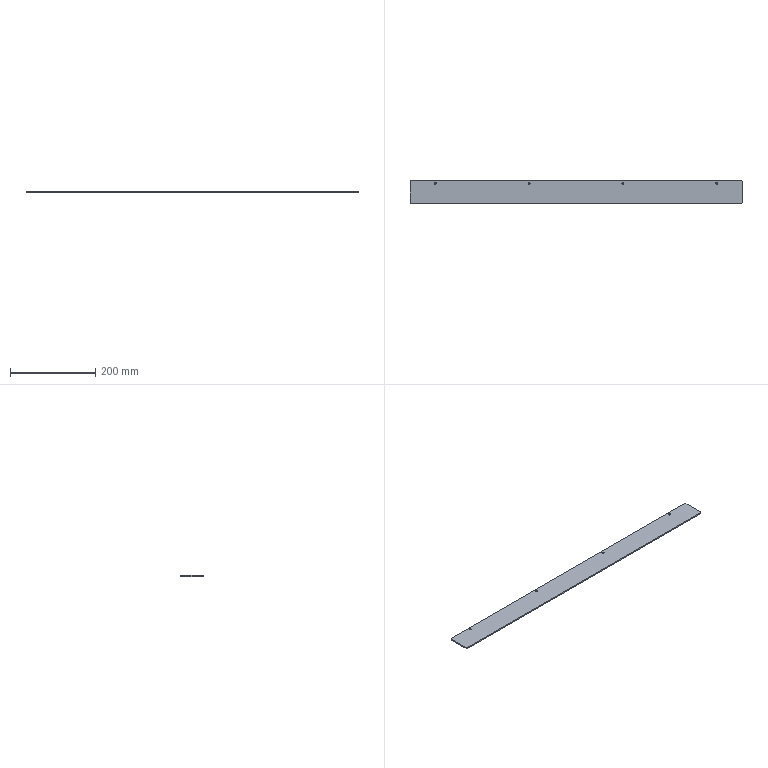Part | NX | features BREP 1 | 1 solid | 26 faces | box 778 x 53 x 3 mm | volume 123272 mm3 | plane 10 | cone 8 | cylinder 8 | commonest cylinder face diameters 4.8 x8
STEP:
#1=CARTESIAN_POINT('',(389.,24.5,3.));
#2=VERTEX_POINT('',#1);
#3=CARTESIAN_POINT('',(387.,26.5,3.));
#4=VERTEX_POINT('',#3);
#5=CARTESIAN_POINT('',(206.75,206.75,3.));
#6=DIRECTION('',(-0.7071,0.7071,0.));
#7=VECTOR('',#6,1000.);
#8=LINE('',#5,#7);
#9=EDGE_CURVE('',#2,#4,#8,.T.);
#10=ORIENTED_EDGE('',*,*,#9,.F.);
#11=CARTESIAN_POINT('',(389.,24.5,0.));
#12=VERTEX_POINT('',#11);
#13=CARTESIAN_POINT('',(389.,24.5,3.));
#14=DIRECTION('',(0.,0.,1.));
#15=VECTOR('',#14,1000.);
#16=LINE('',#13,#15);
#17=EDGE_CURVE('',#12,#2,#16,.T.);
#18=ORIENTED_EDGE('',*,*,#17,.F.);
#19=CARTESIAN_POINT('',(387.,26.5,0.));
#20=VERTEX_POINT('',#19);
#21=CARTESIAN_POINT('',(387.,26.5,0.));
#22=DIRECTION('',(0.7071,-0.7071,0.));
#23=VECTOR('',#22,1000.);
#24=LINE('',#21,#23);
#25=EDGE_CURVE('',#20,#12,#24,.T.);
#26=ORIENTED_EDGE('',*,*,#25,.F.);
#27=CARTESIAN_POINT('',(387.,26.5,3.));
#28=DIRECTION('',(0.,0.,-1.));
#29=VECTOR('',#28,1000.);
#30=LINE('',#27,#29);
#31=EDGE_CURVE('',#4,#20,#30,.T.);
#32=ORIENTED_EDGE('',*,*,#31,.F.);
#33=EDGE_LOOP('',(#10,#18,#26,#32));
#34=FACE_BOUND('',#33,.T.);
#35=CARTESIAN_POINT('',(387.,26.5,3.));
#36=DIRECTION('',(-0.7071,-0.7071,0.));
#37=DIRECTION('',(0.,0.,-1.));
#38=AXIS2_PLACEMENT_3D('',#35,#36,#37);
#39=PLANE('',#38);
#40=ADVANCED_FACE('',(#34),#39,.F.);
#41=CARTESIAN_POINT('',(387.,-26.5,3.));
#42=VERTEX_POINT('',#41);
#43=CARTESIAN_POINT('',(389.,-24.5,3.));
#44=VERTEX_POINT('',#43);
#45=CARTESIAN_POINT('',(206.75,-206.75,3.));
#46=DIRECTION('',(0.7071,0.7071,0.));
#47=VECTOR('',#46,1000.);
#48=LINE('',#45,#47);
#49=EDGE_CURVE('',#42,#44,#48,.T.);
#50=ORIENTED_EDGE('',*,*,#49,.F.);
#51=CARTESIAN_POINT('',(387.,-26.5,0.));
#52=VERTEX_POINT('',#51);
#53=CARTESIAN_POINT('',(387.,-26.5,3.));
#54=DIRECTION('',(0.,0.,1.));
#55=VECTOR('',#54,1000.);
#56=LINE('',#53,#55);
#57=EDGE_CURVE('',#52,#42,#56,.T.);
#58=ORIENTED_EDGE('',*,*,#57,.F.);
#59=CARTESIAN_POINT('',(389.,-24.5,0.));
#60=VERTEX_POINT('',#59);
#61=CARTESIAN_POINT('',(389.,-24.5,0.));
#62=DIRECTION('',(-0.7071,-0.7071,0.));
#63=VECTOR('',#62,1000.);
#64=LINE('',#61,#63);
#65=EDGE_CURVE('',#60,#52,#64,.T.);
#66=ORIENTED_EDGE('',*,*,#65,.F.);
#67=CARTESIAN_POINT('',(389.,-24.5,3.));
#68=DIRECTION('',(0.,0.,-1.));
#69=VECTOR('',#68,1000.);
#70=LINE('',#67,#69);
#71=EDGE_CURVE('',#44,#60,#70,.T.);
#72=ORIENTED_EDGE('',*,*,#71,.F.);
#73=EDGE_LOOP('',(#50,#58,#66,#72));
#74=FACE_BOUND('',#73,.T.);
#75=CARTESIAN_POINT('',(389.,-24.5,3.));
#76=DIRECTION('',(-0.7071,0.7071,0.));
#77=DIRECTION('',(0.,0.,-1.));
#78=AXIS2_PLACEMENT_3D('',#75,#76,#77);
#79=PLANE('',#78);
#80=ADVANCED_FACE('',(#74),#79,.F.);
#81=CARTESIAN_POINT('',(-387.,26.5,3.));
#82=VERTEX_POINT('',#81);
#83=CARTESIAN_POINT('',(-389.,24.5,3.));
#84=VERTEX_POINT('',#83);
#85=CARTESIAN_POINT('',(-206.75,206.75,3.));
#86=DIRECTION('',(-0.7071,-0.7071,0.));
#87=VECTOR('',#86,1000.);
#88=LINE('',#85,#87);
#89=EDGE_CURVE('',#82,#84,#88,.T.);
#90=ORIENTED_EDGE('',*,*,#89,.F.);
#91=CARTESIAN_POINT('',(-387.,26.5,0.));
#92=VERTEX_POINT('',#91);
#93=CARTESIAN_POINT('',(-387.,26.5,3.));
#94=DIRECTION('',(0.,0.,1.));
#95=VECTOR('',#94,1000.);
#96=LINE('',#93,#95);
#97=EDGE_CURVE('',#92,#82,#96,.T.);
#98=ORIENTED_EDGE('',*,*,#97,.F.);
#99=CARTESIAN_POINT('',(-389.,24.5,0.));
#100=VERTEX_POINT('',#99);
#101=CARTESIAN_POINT('',(-389.,24.5,0.));
#102=DIRECTION('',(0.7071,0.7071,0.));
#103=VECTOR('',#102,1000.);
#104=LINE('',#101,#103);
#105=EDGE_CURVE('',#100,#92,#104,.T.);
#106=ORIENTED_EDGE('',*,*,#105,.F.);
#107=CARTESIAN_POINT('',(-389.,24.5,3.));
#108=DIRECTION('',(0.,0.,-1.));
#109=VECTOR('',#108,1000.);
#110=LINE('',#107,#109);
#111=EDGE_CURVE('',#84,#100,#110,.T.);
#112=ORIENTED_EDGE('',*,*,#111,.F.);
#113=EDGE_LOOP('',(#90,#98,#106,#112));
#114=FACE_BOUND('',#113,.T.);
#115=CARTESIAN_POINT('',(-389.,24.5,3.));
#116=DIRECTION('',(0.7071,-0.7071,0.));
#117=DIRECTION('',(0.,0.,-1.));
#118=AXIS2_PLACEMENT_3D('',#115,#116,#117);
#119=PLANE('',#118);
#120=ADVANCED_FACE('',(#114),#119,.F.);
#121=CARTESIAN_POINT('',(-389.,-24.5,3.));
#122=VERTEX_POINT('',#121);
#123=CARTESIAN_POINT('',(-387.,-26.5,3.));
#124=VERTEX_POINT('',#123);
#125=CARTESIAN_POINT('',(-206.75,-206.75,3.));
#126=DIRECTION('',(0.7071,-0.7071,0.));
#127=VECTOR('',#126,1000.);
#128=LINE('',#125,#127);
#129=EDGE_CURVE('',#122,#124,#128,.T.);
#130=ORIENTED_EDGE('',*,*,#129,.F.);
#131=CARTESIAN_POINT('',(-389.,-24.5,0.));
#132=VERTEX_POINT('',#131);
#133=CARTESIAN_POINT('',(-389.,-24.5,3.));
#134=DIRECTION('',(0.,0.,1.));
#135=VECTOR('',#134,1000.);
#136=LINE('',#133,#135);
#137=EDGE_CURVE('',#132,#122,#136,.T.);
#138=ORIENTED_EDGE('',*,*,#137,.F.);
#139=CARTESIAN_POINT('',(-387.,-26.5,0.));
#140=VERTEX_POINT('',#139);
#141=CARTESIAN_POINT('',(-387.,-26.5,0.));
#142=DIRECTION('',(-0.7071,0.7071,0.));
#143=VECTOR('',#142,1000.);
#144=LINE('',#141,#143);
#145=EDGE_CURVE('',#140,#132,#144,.T.);
#146=ORIENTED_EDGE('',*,*,#145,.F.);
#147=CARTESIAN_POINT('',(-387.,-26.5,3.));
#148=DIRECTION('',(0.,0.,-1.));
#149=VECTOR('',#148,1000.);
#150=LINE('',#147,#149);
#151=EDGE_CURVE('',#124,#140,#150,.T.);
#152=ORIENTED_EDGE('',*,*,#151,.F.);
#153=EDGE_LOOP('',(#130,#138,#146,#152));
#154=FACE_BOUND('',#153,.T.);
#155=CARTESIAN_POINT('',(-387.,-26.5,3.));
#156=DIRECTION('',(0.7071,0.7071,0.));
#157=DIRECTION('',(0.,0.,-1.));
#158=AXIS2_PLACEMENT_3D('',#155,#156,#157);
#159=PLANE('',#158);
#160=ADVANCED_FACE('',(#154),#159,.F.);
#161=CARTESIAN_POINT('',(332.4,20.5,2.19));
#162=VERTEX_POINT('',#161);
#163=CARTESIAN_POINT('',(334.59,20.5,0.));
#164=VERTEX_POINT('',#163);
#165=CARTESIAN_POINT('',(334.59,20.5,0.));
#166=DIRECTION('',(0.7071,0.,-0.7071));
#167=VECTOR('',#166,1000.);
#168=LINE('',#165,#167);
#169=EDGE_CURVE('',#162,#164,#168,.T.);
#170=ORIENTED_EDGE('',*,*,#169,.F.);
#171=CARTESIAN_POINT('',(327.6,20.5,2.19));
#172=VERTEX_POINT('',#171);
#173=CARTESIAN_POINT('',(330.,20.5,2.19));
#174=DIRECTION('',(0.,0.,-1.));
#175=DIRECTION('',(-1.,0.,0.));
#176=AXIS2_PLACEMENT_3D('',#173,#174,#175);
#177=CIRCLE('',#176,2.4);
#178=EDGE_CURVE('',#172,#162,#177,.T.);
#179=ORIENTED_EDGE('',*,*,#178,.F.);
#180=CARTESIAN_POINT('',(325.41,20.5,0.));
#181=VERTEX_POINT('',#180);
#182=CARTESIAN_POINT('',(325.41,20.5,0.));
#183=DIRECTION('',(-0.7071,0.,-0.7071));
#184=VECTOR('',#183,1000.);
#185=LINE('',#182,#184);
#186=EDGE_CURVE('',#172,#181,#185,.T.);
#187=ORIENTED_EDGE('',*,*,#186,.T.);
#188=CARTESIAN_POINT('',(330.,20.5,0.));
#189=DIRECTION('',(0.,0.,-1.));
#190=DIRECTION('',(-1.,0.,0.));
#191=AXIS2_PLACEMENT_3D('',#188,#189,#190);
#192=CIRCLE('',#191,4.59);
#193=EDGE_CURVE('',#181,#164,#192,.T.);
#194=ORIENTED_EDGE('',*,*,#193,.T.);
#195=EDGE_LOOP('',(#170,#179,#187,#194));
#196=FACE_BOUND('',#195,.T.);
#197=CARTESIAN_POINT('',(330.,20.5,0.));
#198=DIRECTION('',(0.,0.,-1.));
#199=DIRECTION('',(-1.,0.,0.));
#200=AXIS2_PLACEMENT_3D('',#197,#198,#199);
#201=CONICAL_SURFACE('',#200,4.59,0.7854);
#202=ADVANCED_FACE('',(#196),#201,.F.);
#203=CARTESIAN_POINT('',(332.4,20.5,3.));
#204=VERTEX_POINT('',#203);
#205=CARTESIAN_POINT('',(332.4,20.5,0.));
#206=DIRECTION('',(0.,0.,-1.));
#207=VECTOR('',#206,1000.);
#208=LINE('',#205,#207);
#209=EDGE_CURVE('',#204,#162,#208,.T.);
#210=ORIENTED_EDGE('',*,*,#209,.F.);
#211=CARTESIAN_POINT('',(327.6,20.5,3.));
#212=VERTEX_POINT('',#211);
#213=CARTESIAN_POINT('',(330.,20.5,3.));
#214=DIRECTION('',(0.,0.,-1.));
#215=DIRECTION('',(-1.,0.,0.));
#216=AXIS2_PLACEMENT_3D('',#213,#214,#215);
#217=CIRCLE('',#216,2.4);
#218=EDGE_CURVE('',#212,#204,#217,.T.);
#219=ORIENTED_EDGE('',*,*,#218,.F.);
#220=CARTESIAN_POINT('',(327.6,20.5,0.));
#221=DIRECTION('',(0.,0.,-1.));
#222=VECTOR('',#221,1000.);
#223=LINE('',#220,#222);
#224=EDGE_CURVE('',#212,#172,#223,.T.);
#225=ORIENTED_EDGE('',*,*,#224,.T.);
#226=ORIENTED_EDGE('',*,*,#178,.T.);
#227=EDGE_LOOP('',(#210,#219,#225,#226));
#228=FACE_BOUND('',#227,.T.);
#229=CARTESIAN_POINT('',(330.,20.5,0.));
#230=DIRECTION('',(0.,0.,-1.));
#231=DIRECTION('',(-1.,0.,0.));
#232=AXIS2_PLACEMENT_3D('',#229,#230,#231);
#233=CYLINDRICAL_SURFACE('',#232,2.4);
#234=ADVANCED_FACE('',(#228),#233,.F.);
#235=CARTESIAN_POINT('',(112.4,20.5,2.19));
#236=VERTEX_POINT('',#235);
#237=CARTESIAN_POINT('',(114.59,20.5,0.));
#238=VERTEX_POINT('',#237);
#239=CARTESIAN_POINT('',(114.59,20.5,0.));
#240=DIRECTION('',(0.7071,0.,-0.7071));
#241=VECTOR('',#240,1000.);
#242=LINE('',#239,#241);
#243=EDGE_CURVE('',#236,#238,#242,.T.);
#244=ORIENTED_EDGE('',*,*,#243,.F.);
#245=CARTESIAN_POINT('',(107.6,20.5,2.19));
#246=VERTEX_POINT('',#245);
#247=CARTESIAN_POINT('',(110.,20.5,2.19));
#248=DIRECTION('',(0.,0.,-1.));
#249=DIRECTION('',(-1.,0.,0.));
#250=AXIS2_PLACEMENT_3D('',#247,#248,#249);
#251=CIRCLE('',#250,2.4);
#252=EDGE_CURVE('',#246,#236,#251,.T.);
#253=ORIENTED_EDGE('',*,*,#252,.F.);
#254=CARTESIAN_POINT('',(105.41,20.5,0.));
#255=VERTEX_POINT('',#254);
#256=CARTESIAN_POINT('',(105.41,20.5,0.));
#257=DIRECTION('',(-0.7071,0.,-0.7071));
#258=VECTOR('',#257,1000.);
#259=LINE('',#256,#258);
#260=EDGE_CURVE('',#246,#255,#259,.T.);
#261=ORIENTED_EDGE('',*,*,#260,.T.);
#262=CARTESIAN_POINT('',(110.,20.5,0.));
#263=DIRECTION('',(0.,0.,-1.));
#264=DIRECTION('',(-1.,0.,0.));
#265=AXIS2_PLACEMENT_3D('',#262,#263,#264);
#266=CIRCLE('',#265,4.59);
#267=EDGE_CURVE('',#255,#238,#266,.T.);
#268=ORIENTED_EDGE('',*,*,#267,.T.);
#269=EDGE_LOOP('',(#244,#253,#261,#268));
#270=FACE_BOUND('',#269,.T.);
#271=CARTESIAN_POINT('',(110.,20.5,0.));
#272=DIRECTION('',(0.,0.,-1.));
#273=DIRECTION('',(-1.,0.,0.));
#274=AXIS2_PLACEMENT_3D('',#271,#272,#273);
#275=CONICAL_SURFACE('',#274,4.59,0.7854);
#276=ADVANCED_FACE('',(#270),#275,.F.);
#277=CARTESIAN_POINT('',(112.4,20.5,3.));
#278=VERTEX_POINT('',#277);
#279=CARTESIAN_POINT('',(112.4,20.5,0.));
#280=DIRECTION('',(0.,0.,-1.));
#281=VECTOR('',#280,1000.);
#282=LINE('',#279,#281);
#283=EDGE_CURVE('',#278,#236,#282,.T.);
#284=ORIENTED_EDGE('',*,*,#283,.F.);
#285=CARTESIAN_POINT('',(107.6,20.5,3.));
#286=VERTEX_POINT('',#285);
#287=CARTESIAN_POINT('',(110.,20.5,3.));
#288=DIRECTION('',(0.,0.,-1.));
#289=DIRECTION('',(-1.,0.,0.));
#290=AXIS2_PLACEMENT_3D('',#287,#288,#289);
#291=CIRCLE('',#290,2.4);
#292=EDGE_CURVE('',#286,#278,#291,.T.);
#293=ORIENTED_EDGE('',*,*,#292,.F.);
#294=CARTESIAN_POINT('',(107.6,20.5,0.));
#295=DIRECTION('',(0.,0.,-1.));
#296=VECTOR('',#295,1000.);
#297=LINE('',#294,#296);
#298=EDGE_CURVE('',#286,#246,#297,.T.);
#299=ORIENTED_EDGE('',*,*,#298,.T.);
#300=ORIENTED_EDGE('',*,*,#252,.T.);
#301=EDGE_LOOP('',(#284,#293,#299,#300));
#302=FACE_BOUND('',#301,.T.);
#303=CARTESIAN_POINT('',(110.,20.5,0.));
#304=DIRECTION('',(0.,0.,-1.));
#305=DIRECTION('',(-1.,0.,0.));
#306=AXIS2_PLACEMENT_3D('',#303,#304,#305);
#307=CYLINDRICAL_SURFACE('',#306,2.4);
#308=ADVANCED_FACE('',(#302),#307,.F.);
#309=CARTESIAN_POINT('',(-107.6,20.5,2.19));
#310=VERTEX_POINT('',#309);
#311=CARTESIAN_POINT('',(-105.41,20.5,0.));
#312=VERTEX_POINT('',#311);
#313=CARTESIAN_POINT('',(-105.41,20.5,0.));
#314=DIRECTION('',(0.7071,0.,-0.7071));
#315=VECTOR('',#314,1000.);
#316=LINE('',#313,#315);
#317=EDGE_CURVE('',#310,#312,#316,.T.);
#318=ORIENTED_EDGE('',*,*,#317,.F.);
#319=CARTESIAN_POINT('',(-112.4,20.5,2.19));
#320=VERTEX_POINT('',#319);
#321=CARTESIAN_POINT('',(-110.,20.5,2.19));
#322=DIRECTION('',(0.,0.,-1.));
#323=DIRECTION('',(-1.,0.,0.));
#324=AXIS2_PLACEMENT_3D('',#321,#322,#323);
#325=CIRCLE('',#324,2.4);
#326=EDGE_CURVE('',#320,#310,#325,.T.);
#327=ORIENTED_EDGE('',*,*,#326,.F.);
#328=CARTESIAN_POINT('',(-114.59,20.5,0.));
#329=VERTEX_POINT('',#328);
#330=CARTESIAN_POINT('',(-114.59,20.5,0.));
#331=DIRECTION('',(-0.7071,0.,-0.7071));
#332=VECTOR('',#331,1000.);
#333=LINE('',#330,#332);
#334=EDGE_CURVE('',#320,#329,#333,.T.);
#335=ORIENTED_EDGE('',*,*,#334,.T.);
#336=CARTESIAN_POINT('',(-110.,20.5,0.));
#337=DIRECTION('',(0.,0.,-1.));
#338=DIRECTION('',(-1.,0.,0.));
#339=AXIS2_PLACEMENT_3D('',#336,#337,#338);
#340=CIRCLE('',#339,4.59);
#341=EDGE_CURVE('',#329,#312,#340,.T.);
#342=ORIENTED_EDGE('',*,*,#341,.T.);
#343=EDGE_LOOP('',(#318,#327,#335,#342));
#344=FACE_BOUND('',#343,.T.);
#345=CARTESIAN_POINT('',(-110.,20.5,0.));
#346=DIRECTION('',(0.,0.,-1.));
#347=DIRECTION('',(-1.,0.,0.));
#348=AXIS2_PLACEMENT_3D('',#345,#346,#347);
#349=CONICAL_SURFACE('',#348,4.59,0.7854);
#350=ADVANCED_FACE('',(#344),#349,.F.);
#351=CARTESIAN_POINT('',(-107.6,20.5,3.));
#352=VERTEX_POINT('',#351);
#353=CARTESIAN_POINT('',(-107.6,20.5,0.));
#354=DIRECTION('',(0.,0.,-1.));
#355=VECTOR('',#354,1000.);
#356=LINE('',#353,#355);
#357=EDGE_CURVE('',#352,#310,#356,.T.);
#358=ORIENTED_EDGE('',*,*,#357,.F.);
#359=CARTESIAN_POINT('',(-112.4,20.5,3.));
#360=VERTEX_POINT('',#359);
#361=CARTESIAN_POINT('',(-110.,20.5,3.));
#362=DIRECTION('',(0.,0.,-1.));
#363=DIRECTION('',(-1.,0.,0.));
#364=AXIS2_PLACEMENT_3D('',#361,#362,#363);
#365=CIRCLE('',#364,2.4);
#366=EDGE_CURVE('',#360,#352,#365,.T.);
#367=ORIENTED_EDGE('',*,*,#366,.F.);
#368=CARTESIAN_POINT('',(-112.4,20.5,0.));
#369=DIRECTION('',(0.,0.,-1.));
#370=VECTOR('',#369,1000.);
#371=LINE('',#368,#370);
#372=EDGE_CURVE('',#360,#320,#371,.T.);
#373=ORIENTED_EDGE('',*,*,#372,.T.);
#374=ORIENTED_EDGE('',*,*,#326,.T.);
#375=EDGE_LOOP('',(#358,#367,#373,#374));
#376=FACE_BOUND('',#375,.T.);
#377=CARTESIAN_POINT('',(-110.,20.5,0.));
#378=DIRECTION('',(0.,0.,-1.));
#379=DIRECTION('',(-1.,0.,0.));
#380=AXIS2_PLACEMENT_3D('',#377,#378,#379);
#381=CYLINDRICAL_SURFACE('',#380,2.4);
#382=ADVANCED_FACE('',(#376),#381,.F.);
#383=CARTESIAN_POINT('',(-327.6,20.5,2.19));
#384=VERTEX_POINT('',#383);
#385=CARTESIAN_POINT('',(-325.41,20.5,0.));
#386=VERTEX_POINT('',#385);
#387=CARTESIAN_POINT('',(-325.41,20.5,0.));
#388=DIRECTION('',(0.7071,0.,-0.7071));
#389=VECTOR('',#388,1000.);
#390=LINE('',#387,#389);
#391=EDGE_CURVE('',#384,#386,#390,.T.);
#392=ORIENTED_EDGE('',*,*,#391,.F.);
#393=CARTESIAN_POINT('',(-332.4,20.5,2.19));
#394=VERTEX_POINT('',#393);
#395=CARTESIAN_POINT('',(-330.,20.5,2.19));
#396=DIRECTION('',(0.,0.,-1.));
#397=DIRECTION('',(-1.,0.,0.));
#398=AXIS2_PLACEMENT_3D('',#395,#396,#397);
#399=CIRCLE('',#398,2.4);
#400=EDGE_CURVE('',#394,#384,#399,.T.);
#401=ORIENTED_EDGE('',*,*,#400,.F.);
#402=CARTESIAN_POINT('',(-334.59,20.5,0.));
#403=VERTEX_POINT('',#402);
#404=CARTESIAN_POINT('',(-334.59,20.5,0.));
#405=DIRECTION('',(-0.7071,0.,-0.7071));
#406=VECTOR('',#405,1000.);
#407=LINE('',#404,#406);
#408=EDGE_CURVE('',#394,#403,#407,.T.);
#409=ORIENTED_EDGE('',*,*,#408,.T.);
#410=CARTESIAN_POINT('',(-330.,20.5,0.));
#411=DIRECTION('',(0.,0.,-1.));
#412=DIRECTION('',(-1.,0.,0.));
#413=AXIS2_PLACEMENT_3D('',#410,#411,#412);
#414=CIRCLE('',#413,4.59);
#415=EDGE_CURVE('',#403,#386,#414,.T.);
#416=ORIENTED_EDGE('',*,*,#415,.T.);
#417=EDGE_LOOP('',(#392,#401,#409,#416));
#418=FACE_BOUND('',#417,.T.);
#419=CARTESIAN_POINT('',(-330.,20.5,0.));
#420=DIRECTION('',(0.,0.,-1.));
#421=DIRECTION('',(-1.,0.,0.));
#422=AXIS2_PLACEMENT_3D('',#419,#420,#421);
#423=CONICAL_SURFACE('',#422,4.59,0.7854);
#424=ADVANCED_FACE('',(#418),#423,.F.);
#425=CARTESIAN_POINT('',(-327.6,20.5,3.));
#426=VERTEX_POINT('',#425);
#427=CARTESIAN_POINT('',(-327.6,20.5,0.));
#428=DIRECTION('',(0.,0.,-1.));
#429=VECTOR('',#428,1000.);
#430=LINE('',#427,#429);
#431=EDGE_CURVE('',#426,#384,#430,.T.);
#432=ORIENTED_EDGE('',*,*,#431,.F.);
#433=CARTESIAN_POINT('',(-332.4,20.5,3.));
#434=VERTEX_POINT('',#433);
#435=CARTESIAN_POINT('',(-330.,20.5,3.));
#436=DIRECTION('',(0.,0.,-1.));
#437=DIRECTION('',(-1.,0.,0.));
#438=AXIS2_PLACEMENT_3D('',#435,#436,#437);
#439=CIRCLE('',#438,2.4);
#440=EDGE_CURVE('',#434,#426,#439,.T.);
#441=ORIENTED_EDGE('',*,*,#440,.F.);
#442=CARTESIAN_POINT('',(-332.4,20.5,0.));
#443=DIRECTION('',(0.,0.,-1.));
#444=VECTOR('',#443,1000.);
#445=LINE('',#442,#444);
#446=EDGE_CURVE('',#434,#394,#445,.T.);
#447=ORIENTED_EDGE('',*,*,#446,.T.);
#448=ORIENTED_EDGE('',*,*,#400,.T.);
#449=EDGE_LOOP('',(#432,#441,#447,#448));
#450=FACE_BOUND('',#449,.T.);
#451=CARTESIAN_POINT('',(-330.,20.5,0.));
#452=DIRECTION('',(0.,0.,-1.));
#453=DIRECTION('',(-1.,0.,0.));
#454=AXIS2_PLACEMENT_3D('',#451,#452,#453);
#455=CYLINDRICAL_SURFACE('',#454,2.4);
#456=ADVANCED_FACE('',(#450),#455,.F.);
#457=CARTESIAN_POINT('',(389.,-26.5,0.));
#458=DIRECTION('',(1.,0.,0.));
#459=VECTOR('',#458,1000.);
#460=LINE('',#457,#459);
#461=EDGE_CURVE('',#140,#52,#460,.T.);
#462=ORIENTED_EDGE('',*,*,#461,.F.);
#463=ORIENTED_EDGE('',*,*,#145,.T.);
#464=CARTESIAN_POINT('',(-389.,-26.5,0.));
#465=DIRECTION('',(0.,-1.,0.));
#466=VECTOR('',#465,1000.);
#467=LINE('',#464,#466);
#468=EDGE_CURVE('',#100,#132,#467,.T.);
#469=ORIENTED_EDGE('',*,*,#468,.F.);
#470=ORIENTED_EDGE('',*,*,#105,.T.);
#471=CARTESIAN_POINT('',(389.,26.5,0.));
#472=DIRECTION('',(-1.,0.,0.));
#473=VECTOR('',#472,1000.);
#474=LINE('',#471,#473);
#475=EDGE_CURVE('',#20,#92,#474,.T.);
#476=ORIENTED_EDGE('',*,*,#475,.F.);
#477=ORIENTED_EDGE('',*,*,#25,.T.);
#478=CARTESIAN_POINT('',(389.,-26.5,0.));
#479=DIRECTION('',(0.,1.,0.));
#480=VECTOR('',#479,1000.);
#481=LINE('',#478,#480);
#482=EDGE_CURVE('',#60,#12,#481,.T.);
#483=ORIENTED_EDGE('',*,*,#482,.F.);
#484=ORIENTED_EDGE('',*,*,#65,.T.);
#485=EDGE_LOOP('',(#462,#463,#469,#470,#476,#477,#483,#484));
#486=FACE_BOUND('',#485,.T.);
#487=ORIENTED_EDGE('',*,*,#415,.F.);
#488=CARTESIAN_POINT('',(-330.,20.5,0.));
#489=DIRECTION('',(0.,0.,-1.));
#490=DIRECTION('',(-1.,0.,0.));
#491=AXIS2_PLACEMENT_3D('',#488,#489,#490);
#492=CIRCLE('',#491,4.59);
#493=EDGE_CURVE('',#386,#403,#492,.T.);
#494=ORIENTED_EDGE('',*,*,#493,.F.);
#495=EDGE_LOOP('',(#487,#494));
#496=FACE_BOUND('',#495,.T.);
#497=ORIENTED_EDGE('',*,*,#341,.F.);
#498=CARTESIAN_POINT('',(-110.,20.5,0.));
#499=DIRECTION('',(0.,0.,-1.));
#500=DIRECTION('',(-1.,0.,0.));
#501=AXIS2_PLACEMENT_3D('',#498,#499,#500);
#502=CIRCLE('',#501,4.59);
#503=EDGE_CURVE('',#312,#329,#502,.T.);
#504=ORIENTED_EDGE('',*,*,#503,.F.);
#505=EDGE_LOOP('',(#497,#504));
#506=FACE_BOUND('',#505,.T.);
#507=ORIENTED_EDGE('',*,*,#267,.F.);
#508=CARTESIAN_POINT('',(110.,20.5,0.));
#509=DIRECTION('',(0.,0.,-1.));
#510=DIRECTION('',(-1.,0.,0.));
#511=AXIS2_PLACEMENT_3D('',#508,#509,#510);
#512=CIRCLE('',#511,4.59);
#513=EDGE_CURVE('',#238,#255,#512,.T.);
#514=ORIENTED_EDGE('',*,*,#513,.F.);
#515=EDGE_LOOP('',(#507,#514));
#516=FACE_BOUND('',#515,.T.);
#517=ORIENTED_EDGE('',*,*,#193,.F.);
#518=CARTESIAN_POINT('',(330.,20.5,0.));
#519=DIRECTION('',(0.,0.,-1.));
#520=DIRECTION('',(-1.,0.,0.));
#521=AXIS2_PLACEMENT_3D('',#518,#519,#520);
#522=CIRCLE('',#521,4.59);
#523=EDGE_CURVE('',#164,#181,#522,.T.);
#524=ORIENTED_EDGE('',*,*,#523,.F.);
#525=EDGE_LOOP('',(#517,#524));
#526=FACE_BOUND('',#525,.T.);
#527=CARTESIAN_POINT('',(0.,0.,0.));
#528=DIRECTION('',(0.,0.,1.));
#529=DIRECTION('',(1.,0.,0.));
#530=AXIS2_PLACEMENT_3D('',#527,#528,#529);
#531=PLANE('',#530);
#532=ADVANCED_FACE('',(#486,#496,#506,#516,#526),#531,.F.);
#533=CARTESIAN_POINT('',(-389.,-26.5,3.));
#534=DIRECTION('',(0.,-1.,0.));
#535=VECTOR('',#534,1000.);
#536=LINE('',#533,#535);
#537=EDGE_CURVE('',#84,#122,#536,.T.);
#538=ORIENTED_EDGE('',*,*,#537,.T.);
#539=ORIENTED_EDGE('',*,*,#129,.T.);
#540=CARTESIAN_POINT('',(389.,-26.5,3.));
#541=DIRECTION('',(1.,0.,0.));
#542=VECTOR('',#541,1000.);
#543=LINE('',#540,#542);
#544=EDGE_CURVE('',#124,#42,#543,.T.);
#545=ORIENTED_EDGE('',*,*,#544,.T.);
#546=ORIENTED_EDGE('',*,*,#49,.T.);
#547=CARTESIAN_POINT('',(389.,-26.5,3.));
#548=DIRECTION('',(0.,1.,0.));
#549=VECTOR('',#548,1000.);
#550=LINE('',#547,#549);
#551=EDGE_CURVE('',#44,#2,#550,.T.);
#552=ORIENTED_EDGE('',*,*,#551,.T.);
#553=ORIENTED_EDGE('',*,*,#9,.T.);
#554=CARTESIAN_POINT('',(389.,26.5,3.));
#555=DIRECTION('',(-1.,0.,0.));
#556=VECTOR('',#555,1000.);
#557=LINE('',#554,#556);
#558=EDGE_CURVE('',#4,#82,#557,.T.);
#559=ORIENTED_EDGE('',*,*,#558,.T.);
#560=ORIENTED_EDGE('',*,*,#89,.T.);
#561=EDGE_LOOP('',(#538,#539,#545,#546,#552,#553,#559,#560));
#562=FACE_BOUND('',#561,.T.);
#563=ORIENTED_EDGE('',*,*,#440,.T.);
#564=CARTESIAN_POINT('',(-330.,20.5,3.));
#565=DIRECTION('',(0.,0.,-1.));
#566=DIRECTION('',(-1.,0.,0.));
#567=AXIS2_PLACEMENT_3D('',#564,#565,#566);
#568=CIRCLE('',#567,2.4);
#569=EDGE_CURVE('',#426,#434,#568,.T.);
#570=ORIENTED_EDGE('',*,*,#569,.T.);
#571=EDGE_LOOP('',(#563,#570));
#572=FACE_BOUND('',#571,.T.);
#573=ORIENTED_EDGE('',*,*,#366,.T.);
#574=CARTESIAN_POINT('',(-110.,20.5,3.));
#575=DIRECTION('',(0.,0.,-1.));
#576=DIRECTION('',(-1.,0.,0.));
#577=AXIS2_PLACEMENT_3D('',#574,#575,#576);
#578=CIRCLE('',#577,2.4);
#579=EDGE_CURVE('',#352,#360,#578,.T.);
#580=ORIENTED_EDGE('',*,*,#579,.T.);
#581=EDGE_LOOP('',(#573,#580));
#582=FACE_BOUND('',#581,.T.);
#583=ORIENTED_EDGE('',*,*,#292,.T.);
#584=CARTESIAN_POINT('',(110.,20.5,3.));
#585=DIRECTION('',(0.,0.,-1.));
#586=DIRECTION('',(-1.,0.,0.));
#587=AXIS2_PLACEMENT_3D('',#584,#585,#586);
#588=CIRCLE('',#587,2.4);
#589=EDGE_CURVE('',#278,#286,#588,.T.);
#590=ORIENTED_EDGE('',*,*,#589,.T.);
#591=EDGE_LOOP('',(#583,#590));
#592=FACE_BOUND('',#591,.T.);
#593=ORIENTED_EDGE('',*,*,#218,.T.);
#594=CARTESIAN_POINT('',(330.,20.5,3.));
#595=DIRECTION('',(0.,0.,-1.));
#596=DIRECTION('',(-1.,0.,0.));
#597=AXIS2_PLACEMENT_3D('',#594,#595,#596);
#598=CIRCLE('',#597,2.4);
#599=EDGE_CURVE('',#204,#212,#598,.T.);
#600=ORIENTED_EDGE('',*,*,#599,.T.);
#601=EDGE_LOOP('',(#593,#600));
#602=FACE_BOUND('',#601,.T.);
#603=CARTESIAN_POINT('',(0.,0.,3.));
#604=DIRECTION('',(0.,0.,1.));
#605=DIRECTION('',(1.,0.,0.));
#606=AXIS2_PLACEMENT_3D('',#603,#604,#605);
#607=PLANE('',#606);
#608=ADVANCED_FACE('',(#562,#572,#582,#592,#602),#607,.T.);
#609=ORIENTED_EDGE('',*,*,#475,.T.);
#610=ORIENTED_EDGE('',*,*,#97,.T.);
#611=ORIENTED_EDGE('',*,*,#558,.F.);
#612=ORIENTED_EDGE('',*,*,#31,.T.);
#613=EDGE_LOOP('',(#609,#610,#611,#612));
#614=FACE_BOUND('',#613,.T.);
#615=CARTESIAN_POINT('',(389.,26.5,3.));
#616=DIRECTION('',(0.,-1.,0.));
#617=DIRECTION('',(1.,0.,0.));
#618=AXIS2_PLACEMENT_3D('',#615,#616,#617);
#619=PLANE('',#618);
#620=ADVANCED_FACE('',(#614),#619,.F.);
#621=ORIENTED_EDGE('',*,*,#551,.F.);
#622=ORIENTED_EDGE('',*,*,#71,.T.);
#623=ORIENTED_EDGE('',*,*,#482,.T.);
#624=ORIENTED_EDGE('',*,*,#17,.T.);
#625=EDGE_LOOP('',(#621,#622,#623,#624));
#626=FACE_BOUND('',#625,.T.);
#627=CARTESIAN_POINT('',(389.,-26.5,3.));
#628=DIRECTION('',(-1.,0.,0.));
#629=DIRECTION('',(0.,0.,1.));
#630=AXIS2_PLACEMENT_3D('',#627,#628,#629);
#631=PLANE('',#630);
#632=ADVANCED_FACE('',(#626),#631,.F.);
#633=ORIENTED_EDGE('',*,*,#544,.F.);
#634=ORIENTED_EDGE('',*,*,#151,.T.);
#635=ORIENTED_EDGE('',*,*,#461,.T.);
#636=ORIENTED_EDGE('',*,*,#57,.T.);
#637=EDGE_LOOP('',(#633,#634,#635,#636));
#638=FACE_BOUND('',#637,.T.);
#639=CARTESIAN_POINT('',(389.,-26.5,3.));
#640=DIRECTION('',(0.,1.,0.));
#641=DIRECTION('',(-1.,0.,0.));
#642=AXIS2_PLACEMENT_3D('',#639,#640,#641);
#643=PLANE('',#642);
#644=ADVANCED_FACE('',(#638),#643,.F.);
#645=ORIENTED_EDGE('',*,*,#468,.T.);
#646=ORIENTED_EDGE('',*,*,#137,.T.);
#647=ORIENTED_EDGE('',*,*,#537,.F.);
#648=ORIENTED_EDGE('',*,*,#111,.T.);
#649=EDGE_LOOP('',(#645,#646,#647,#648));
#650=FACE_BOUND('',#649,.T.);
#651=CARTESIAN_POINT('',(-389.,-26.5,3.));
#652=DIRECTION('',(1.,0.,0.));
#653=DIRECTION('',(0.,0.,-1.));
#654=AXIS2_PLACEMENT_3D('',#651,#652,#653);
#655=PLANE('',#654);
#656=ADVANCED_FACE('',(#650),#655,.F.);
#657=ORIENTED_EDGE('',*,*,#569,.F.);
#658=ORIENTED_EDGE('',*,*,#431,.T.);
#659=CARTESIAN_POINT('',(-330.,20.5,2.19));
#660=DIRECTION('',(0.,0.,-1.));
#661=DIRECTION('',(-1.,0.,0.));
#662=AXIS2_PLACEMENT_3D('',#659,#660,#661);
#663=CIRCLE('',#662,2.4);
#664=EDGE_CURVE('',#384,#394,#663,.T.);
#665=ORIENTED_EDGE('',*,*,#664,.T.);
#666=ORIENTED_EDGE('',*,*,#446,.F.);
#667=EDGE_LOOP('',(#657,#658,#665,#666));
#668=FACE_BOUND('',#667,.T.);
#669=CARTESIAN_POINT('',(-330.,20.5,0.));
#670=DIRECTION('',(0.,0.,-1.));
#671=DIRECTION('',(-1.,0.,0.));
#672=AXIS2_PLACEMENT_3D('',#669,#670,#671);
#673=CYLINDRICAL_SURFACE('',#672,2.4);
#674=ADVANCED_FACE('',(#668),#673,.F.);
#675=ORIENTED_EDGE('',*,*,#664,.F.);
#676=ORIENTED_EDGE('',*,*,#391,.T.);
#677=ORIENTED_EDGE('',*,*,#493,.T.);
#678=ORIENTED_EDGE('',*,*,#408,.F.);
#679=EDGE_LOOP('',(#675,#676,#677,#678));
#680=FACE_BOUND('',#679,.T.);
#681=CARTESIAN_POINT('',(-330.,20.5,0.));
#682=DIRECTION('',(0.,0.,-1.));
#683=DIRECTION('',(-1.,0.,0.));
#684=AXIS2_PLACEMENT_3D('',#681,#682,#683);
#685=CONICAL_SURFACE('',#684,4.59,0.7854);
#686=ADVANCED_FACE('',(#680),#685,.F.);
#687=ORIENTED_EDGE('',*,*,#579,.F.);
#688=ORIENTED_EDGE('',*,*,#357,.T.);
#689=CARTESIAN_POINT('',(-110.,20.5,2.19));
#690=DIRECTION('',(0.,0.,-1.));
#691=DIRECTION('',(-1.,0.,0.));
#692=AXIS2_PLACEMENT_3D('',#689,#690,#691);
#693=CIRCLE('',#692,2.4);
#694=EDGE_CURVE('',#310,#320,#693,.T.);
#695=ORIENTED_EDGE('',*,*,#694,.T.);
#696=ORIENTED_EDGE('',*,*,#372,.F.);
#697=EDGE_LOOP('',(#687,#688,#695,#696));
#698=FACE_BOUND('',#697,.T.);
#699=CARTESIAN_POINT('',(-110.,20.5,0.));
#700=DIRECTION('',(0.,0.,-1.));
#701=DIRECTION('',(-1.,0.,0.));
#702=AXIS2_PLACEMENT_3D('',#699,#700,#701);
#703=CYLINDRICAL_SURFACE('',#702,2.4);
#704=ADVANCED_FACE('',(#698),#703,.F.);
#705=ORIENTED_EDGE('',*,*,#694,.F.);
#706=ORIENTED_EDGE('',*,*,#317,.T.);
#707=ORIENTED_EDGE('',*,*,#503,.T.);
#708=ORIENTED_EDGE('',*,*,#334,.F.);
#709=EDGE_LOOP('',(#705,#706,#707,#708));
#710=FACE_BOUND('',#709,.T.);
#711=CARTESIAN_POINT('',(-110.,20.5,0.));
#712=DIRECTION('',(0.,0.,-1.));
#713=DIRECTION('',(-1.,0.,0.));
#714=AXIS2_PLACEMENT_3D('',#711,#712,#713);
#715=CONICAL_SURFACE('',#714,4.59,0.7854);
#716=ADVANCED_FACE('',(#710),#715,.F.);
#717=ORIENTED_EDGE('',*,*,#589,.F.);
#718=ORIENTED_EDGE('',*,*,#283,.T.);
#719=CARTESIAN_POINT('',(110.,20.5,2.19));
#720=DIRECTION('',(0.,0.,-1.));
#721=DIRECTION('',(-1.,0.,0.));
#722=AXIS2_PLACEMENT_3D('',#719,#720,#721);
#723=CIRCLE('',#722,2.4);
#724=EDGE_CURVE('',#236,#246,#723,.T.);
#725=ORIENTED_EDGE('',*,*,#724,.T.);
#726=ORIENTED_EDGE('',*,*,#298,.F.);
#727=EDGE_LOOP('',(#717,#718,#725,#726));
#728=FACE_BOUND('',#727,.T.);
#729=CARTESIAN_POINT('',(110.,20.5,0.));
#730=DIRECTION('',(0.,0.,-1.));
#731=DIRECTION('',(-1.,0.,0.));
#732=AXIS2_PLACEMENT_3D('',#729,#730,#731);
#733=CYLINDRICAL_SURFACE('',#732,2.4);
#734=ADVANCED_FACE('',(#728),#733,.F.);
#735=ORIENTED_EDGE('',*,*,#724,.F.);
#736=ORIENTED_EDGE('',*,*,#243,.T.);
#737=ORIENTED_EDGE('',*,*,#513,.T.);
#738=ORIENTED_EDGE('',*,*,#260,.F.);
#739=EDGE_LOOP('',(#735,#736,#737,#738));
#740=FACE_BOUND('',#739,.T.);
#741=CARTESIAN_POINT('',(110.,20.5,0.));
#742=DIRECTION('',(0.,0.,-1.));
#743=DIRECTION('',(-1.,0.,0.));
#744=AXIS2_PLACEMENT_3D('',#741,#742,#743);
#745=CONICAL_SURFACE('',#744,4.59,0.7854);
#746=ADVANCED_FACE('',(#740),#745,.F.);
#747=ORIENTED_EDGE('',*,*,#599,.F.);
#748=ORIENTED_EDGE('',*,*,#209,.T.);
#749=CARTESIAN_POINT('',(330.,20.5,2.19));
#750=DIRECTION('',(0.,0.,-1.));
#751=DIRECTION('',(-1.,0.,0.));
#752=AXIS2_PLACEMENT_3D('',#749,#750,#751);
#753=CIRCLE('',#752,2.4);
#754=EDGE_CURVE('',#162,#172,#753,.T.);
#755=ORIENTED_EDGE('',*,*,#754,.T.);
#756=ORIENTED_EDGE('',*,*,#224,.F.);
#757=EDGE_LOOP('',(#747,#748,#755,#756));
#758=FACE_BOUND('',#757,.T.);
#759=CARTESIAN_POINT('',(330.,20.5,0.));
#760=DIRECTION('',(0.,0.,-1.));
#761=DIRECTION('',(-1.,0.,0.));
#762=AXIS2_PLACEMENT_3D('',#759,#760,#761);
#763=CYLINDRICAL_SURFACE('',#762,2.4);
#764=ADVANCED_FACE('',(#758),#763,.F.);
#765=ORIENTED_EDGE('',*,*,#754,.F.);
#766=ORIENTED_EDGE('',*,*,#169,.T.);
#767=ORIENTED_EDGE('',*,*,#523,.T.);
#768=ORIENTED_EDGE('',*,*,#186,.F.);
#769=EDGE_LOOP('',(#765,#766,#767,#768));
#770=FACE_BOUND('',#769,.T.);
#771=CARTESIAN_POINT('',(330.,20.5,0.));
#772=DIRECTION('',(0.,0.,-1.));
#773=DIRECTION('',(-1.,0.,0.));
#774=AXIS2_PLACEMENT_3D('',#771,#772,#773);
#775=CONICAL_SURFACE('',#774,4.59,0.7854);
#776=ADVANCED_FACE('',(#770),#775,.F.);
#777=CLOSED_SHELL('',(#40,#80,#120,#160,#202,#234,#276,#308,#350,#382,#424,#456,#532,#608,#620,#632,#644,#656,#674,#686,#704,#716,#734,#746,#764,#776));
#778=MANIFOLD_SOLID_BREP('',#777);
#779=(LENGTH_UNIT()NAMED_UNIT(*)SI_UNIT(.MILLI.,.METRE.));
#780=UNCERTAINTY_MEASURE_WITH_UNIT(LENGTH_MEASURE(0.00001),#779,'','');
#781=(NAMED_UNIT(*)PLANE_ANGLE_UNIT()SI_UNIT($,.RADIAN.));
#782=(NAMED_UNIT(*)SI_UNIT($,.STERADIAN.)SOLID_ANGLE_UNIT());
#783=(GEOMETRIC_REPRESENTATION_CONTEXT(3)GLOBAL_UNCERTAINTY_ASSIGNED_CONTEXT((#780))GLOBAL_UNIT_ASSIGNED_CONTEXT((#779,#781,#782))REPRESENTATION_CONTEXT('',''));
#784=ADVANCED_BREP_SHAPE_REPRESENTATION('',(#778),#783);